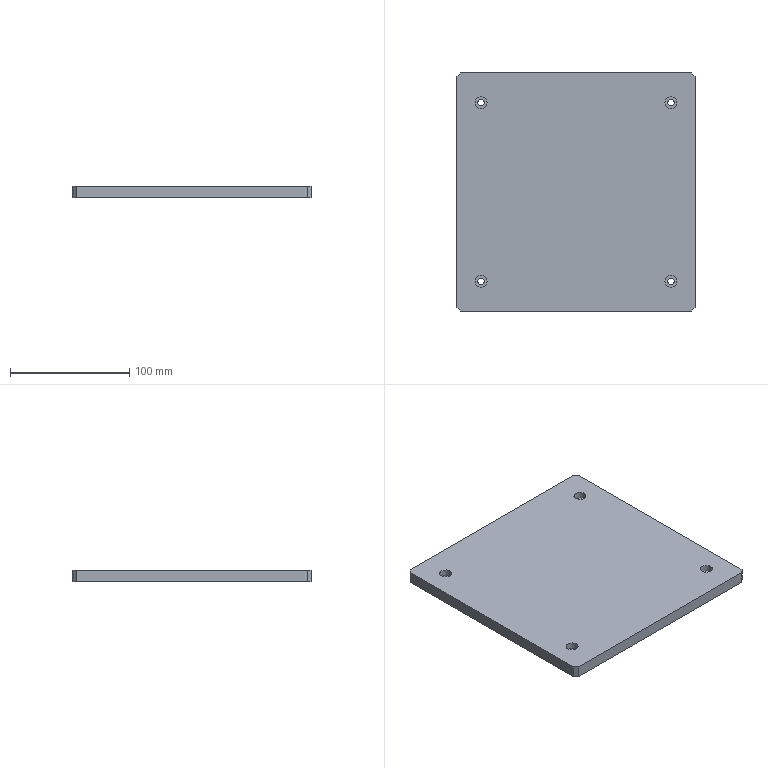Part | SolidWorks | features Chamfer 1, Extrusion 1, HoleWzd 1 | 1 solid | 30 faces | box 200 x 200 x 10 mm | volume 397621 mm3 | cylinder 16 | plane 14 | commonest cylinder face diameters 5.5 x8 10 x8
STEP:
#1=CARTESIAN_POINT('',(-84.68,75.,4.3));
#2=VERTEX_POINT('',#1);
#3=CARTESIAN_POINT('',(-74.68,75.,4.3));
#4=VERTEX_POINT('',#3);
#5=CARTESIAN_POINT('',(-79.68,75.,4.3));
#6=DIRECTION('',(0.,0.,1.));
#7=DIRECTION('',(1.,0.,0.));
#8=AXIS2_PLACEMENT_3D('',#5,#6,#7);
#9=CIRCLE('',#8,5.);
#10=EDGE_CURVE('',#2,#4,#9,.T.);
#11=ORIENTED_EDGE('',*,*,#10,.F.);
#12=CARTESIAN_POINT('',(-84.68,75.,10.));
#13=VERTEX_POINT('',#12);
#14=CARTESIAN_POINT('',(-84.68,75.,10.));
#15=DIRECTION('',(0.,0.,1.));
#16=VECTOR('',#15,1000.);
#17=LINE('',#14,#16);
#18=EDGE_CURVE('',#2,#13,#17,.T.);
#19=ORIENTED_EDGE('',*,*,#18,.T.);
#20=CARTESIAN_POINT('',(-74.68,75.,10.));
#21=VERTEX_POINT('',#20);
#22=CARTESIAN_POINT('',(-79.68,75.,10.));
#23=DIRECTION('',(0.,0.,1.));
#24=DIRECTION('',(1.,0.,0.));
#25=AXIS2_PLACEMENT_3D('',#22,#23,#24);
#26=CIRCLE('',#25,5.);
#27=EDGE_CURVE('',#13,#21,#26,.T.);
#28=ORIENTED_EDGE('',*,*,#27,.T.);
#29=CARTESIAN_POINT('',(-74.68,75.,10.));
#30=DIRECTION('',(0.,0.,1.));
#31=VECTOR('',#30,1000.);
#32=LINE('',#29,#31);
#33=EDGE_CURVE('',#4,#21,#32,.T.);
#34=ORIENTED_EDGE('',*,*,#33,.F.);
#35=EDGE_LOOP('',(#11,#19,#28,#34));
#36=FACE_OUTER_BOUND('',#35,.T.);
#37=CARTESIAN_POINT('',(-79.68,75.,10.));
#38=DIRECTION('',(0.,0.,1.));
#39=DIRECTION('',(1.,0.,0.));
#40=AXIS2_PLACEMENT_3D('',#37,#38,#39);
#41=CYLINDRICAL_SURFACE('',#40,5.);
#42=ADVANCED_FACE('',(#36),#41,.F.);
#43=CARTESIAN_POINT('',(-76.93,75.,0.));
#44=VERTEX_POINT('',#43);
#45=CARTESIAN_POINT('',(-82.43,75.,0.));
#46=VERTEX_POINT('',#45);
#47=CARTESIAN_POINT('',(-79.68,75.,0.));
#48=DIRECTION('',(0.,0.,-1.));
#49=DIRECTION('',(-1.,0.,0.));
#50=AXIS2_PLACEMENT_3D('',#47,#48,#49);
#51=CIRCLE('',#50,2.75);
#52=EDGE_CURVE('',#44,#46,#51,.T.);
#53=ORIENTED_EDGE('',*,*,#52,.T.);
#54=CARTESIAN_POINT('',(-82.43,75.,4.3));
#55=VERTEX_POINT('',#54);
#56=CARTESIAN_POINT('',(-82.43,75.,10.));
#57=DIRECTION('',(0.,0.,1.));
#58=VECTOR('',#57,1000.);
#59=LINE('',#56,#58);
#60=EDGE_CURVE('',#46,#55,#59,.T.);
#61=ORIENTED_EDGE('',*,*,#60,.T.);
#62=CARTESIAN_POINT('',(-76.93,75.,4.3));
#63=VERTEX_POINT('',#62);
#64=CARTESIAN_POINT('',(-79.68,75.,4.3));
#65=DIRECTION('',(0.,0.,1.));
#66=DIRECTION('',(1.,0.,0.));
#67=AXIS2_PLACEMENT_3D('',#64,#65,#66);
#68=CIRCLE('',#67,2.75);
#69=EDGE_CURVE('',#55,#63,#68,.T.);
#70=ORIENTED_EDGE('',*,*,#69,.T.);
#71=CARTESIAN_POINT('',(-76.93,75.,10.));
#72=DIRECTION('',(0.,0.,1.));
#73=VECTOR('',#72,1000.);
#74=LINE('',#71,#73);
#75=EDGE_CURVE('',#44,#63,#74,.T.);
#76=ORIENTED_EDGE('',*,*,#75,.F.);
#77=EDGE_LOOP('',(#53,#61,#70,#76));
#78=FACE_OUTER_BOUND('',#77,.T.);
#79=CARTESIAN_POINT('',(-79.68,75.,10.));
#80=DIRECTION('',(0.,0.,1.));
#81=DIRECTION('',(1.,0.,0.));
#82=AXIS2_PLACEMENT_3D('',#79,#80,#81);
#83=CYLINDRICAL_SURFACE('',#82,2.75);
#84=ADVANCED_FACE('',(#78),#83,.F.);
#85=CARTESIAN_POINT('',(74.68,75.,4.3));
#86=VERTEX_POINT('',#85);
#87=CARTESIAN_POINT('',(84.68,75.,4.3));
#88=VERTEX_POINT('',#87);
#89=CARTESIAN_POINT('',(79.68,75.,4.3));
#90=DIRECTION('',(0.,0.,1.));
#91=DIRECTION('',(1.,0.,0.));
#92=AXIS2_PLACEMENT_3D('',#89,#90,#91);
#93=CIRCLE('',#92,5.);
#94=EDGE_CURVE('',#86,#88,#93,.T.);
#95=ORIENTED_EDGE('',*,*,#94,.F.);
#96=CARTESIAN_POINT('',(74.68,75.,10.));
#97=VERTEX_POINT('',#96);
#98=CARTESIAN_POINT('',(74.68,75.,10.));
#99=DIRECTION('',(0.,0.,1.));
#100=VECTOR('',#99,1000.);
#101=LINE('',#98,#100);
#102=EDGE_CURVE('',#86,#97,#101,.T.);
#103=ORIENTED_EDGE('',*,*,#102,.T.);
#104=CARTESIAN_POINT('',(84.68,75.,10.));
#105=VERTEX_POINT('',#104);
#106=CARTESIAN_POINT('',(79.68,75.,10.));
#107=DIRECTION('',(0.,0.,1.));
#108=DIRECTION('',(1.,0.,0.));
#109=AXIS2_PLACEMENT_3D('',#106,#107,#108);
#110=CIRCLE('',#109,5.);
#111=EDGE_CURVE('',#97,#105,#110,.T.);
#112=ORIENTED_EDGE('',*,*,#111,.T.);
#113=CARTESIAN_POINT('',(84.68,75.,10.));
#114=DIRECTION('',(0.,0.,1.));
#115=VECTOR('',#114,1000.);
#116=LINE('',#113,#115);
#117=EDGE_CURVE('',#88,#105,#116,.T.);
#118=ORIENTED_EDGE('',*,*,#117,.F.);
#119=EDGE_LOOP('',(#95,#103,#112,#118));
#120=FACE_OUTER_BOUND('',#119,.T.);
#121=CARTESIAN_POINT('',(79.68,75.,10.));
#122=DIRECTION('',(0.,0.,1.));
#123=DIRECTION('',(1.,0.,0.));
#124=AXIS2_PLACEMENT_3D('',#121,#122,#123);
#125=CYLINDRICAL_SURFACE('',#124,5.);
#126=ADVANCED_FACE('',(#120),#125,.F.);
#127=CARTESIAN_POINT('',(82.43,75.,0.));
#128=VERTEX_POINT('',#127);
#129=CARTESIAN_POINT('',(76.93,75.,0.));
#130=VERTEX_POINT('',#129);
#131=CARTESIAN_POINT('',(79.68,75.,0.));
#132=DIRECTION('',(0.,0.,-1.));
#133=DIRECTION('',(-1.,0.,0.));
#134=AXIS2_PLACEMENT_3D('',#131,#132,#133);
#135=CIRCLE('',#134,2.75);
#136=EDGE_CURVE('',#128,#130,#135,.T.);
#137=ORIENTED_EDGE('',*,*,#136,.T.);
#138=CARTESIAN_POINT('',(76.93,75.,4.3));
#139=VERTEX_POINT('',#138);
#140=CARTESIAN_POINT('',(76.93,75.,10.));
#141=DIRECTION('',(0.,0.,1.));
#142=VECTOR('',#141,1000.);
#143=LINE('',#140,#142);
#144=EDGE_CURVE('',#130,#139,#143,.T.);
#145=ORIENTED_EDGE('',*,*,#144,.T.);
#146=CARTESIAN_POINT('',(82.43,75.,4.3));
#147=VERTEX_POINT('',#146);
#148=CARTESIAN_POINT('',(79.68,75.,4.3));
#149=DIRECTION('',(0.,0.,1.));
#150=DIRECTION('',(1.,0.,0.));
#151=AXIS2_PLACEMENT_3D('',#148,#149,#150);
#152=CIRCLE('',#151,2.75);
#153=EDGE_CURVE('',#139,#147,#152,.T.);
#154=ORIENTED_EDGE('',*,*,#153,.T.);
#155=CARTESIAN_POINT('',(82.43,75.,10.));
#156=DIRECTION('',(0.,0.,1.));
#157=VECTOR('',#156,1000.);
#158=LINE('',#155,#157);
#159=EDGE_CURVE('',#128,#147,#158,.T.);
#160=ORIENTED_EDGE('',*,*,#159,.F.);
#161=EDGE_LOOP('',(#137,#145,#154,#160));
#162=FACE_OUTER_BOUND('',#161,.T.);
#163=CARTESIAN_POINT('',(79.68,75.,10.));
#164=DIRECTION('',(0.,0.,1.));
#165=DIRECTION('',(1.,0.,0.));
#166=AXIS2_PLACEMENT_3D('',#163,#164,#165);
#167=CYLINDRICAL_SURFACE('',#166,2.75);
#168=ADVANCED_FACE('',(#162),#167,.F.);
#169=CARTESIAN_POINT('',(74.68,-75.,4.3));
#170=VERTEX_POINT('',#169);
#171=CARTESIAN_POINT('',(84.68,-75.,4.3));
#172=VERTEX_POINT('',#171);
#173=CARTESIAN_POINT('',(79.68,-75.,4.3));
#174=DIRECTION('',(0.,0.,1.));
#175=DIRECTION('',(1.,0.,0.));
#176=AXIS2_PLACEMENT_3D('',#173,#174,#175);
#177=CIRCLE('',#176,5.);
#178=EDGE_CURVE('',#170,#172,#177,.T.);
#179=ORIENTED_EDGE('',*,*,#178,.F.);
#180=CARTESIAN_POINT('',(74.68,-75.,10.));
#181=VERTEX_POINT('',#180);
#182=CARTESIAN_POINT('',(74.68,-75.,10.));
#183=DIRECTION('',(0.,0.,1.));
#184=VECTOR('',#183,1000.);
#185=LINE('',#182,#184);
#186=EDGE_CURVE('',#170,#181,#185,.T.);
#187=ORIENTED_EDGE('',*,*,#186,.T.);
#188=CARTESIAN_POINT('',(84.68,-75.,10.));
#189=VERTEX_POINT('',#188);
#190=CARTESIAN_POINT('',(79.68,-75.,10.));
#191=DIRECTION('',(0.,0.,1.));
#192=DIRECTION('',(1.,0.,0.));
#193=AXIS2_PLACEMENT_3D('',#190,#191,#192);
#194=CIRCLE('',#193,5.);
#195=EDGE_CURVE('',#181,#189,#194,.T.);
#196=ORIENTED_EDGE('',*,*,#195,.T.);
#197=CARTESIAN_POINT('',(84.68,-75.,10.));
#198=DIRECTION('',(0.,0.,1.));
#199=VECTOR('',#198,1000.);
#200=LINE('',#197,#199);
#201=EDGE_CURVE('',#172,#189,#200,.T.);
#202=ORIENTED_EDGE('',*,*,#201,.F.);
#203=EDGE_LOOP('',(#179,#187,#196,#202));
#204=FACE_OUTER_BOUND('',#203,.T.);
#205=CARTESIAN_POINT('',(79.68,-75.,10.));
#206=DIRECTION('',(0.,0.,1.));
#207=DIRECTION('',(1.,0.,0.));
#208=AXIS2_PLACEMENT_3D('',#205,#206,#207);
#209=CYLINDRICAL_SURFACE('',#208,5.);
#210=ADVANCED_FACE('',(#204),#209,.F.);
#211=CARTESIAN_POINT('',(82.43,-75.,0.));
#212=VERTEX_POINT('',#211);
#213=CARTESIAN_POINT('',(76.93,-75.,0.));
#214=VERTEX_POINT('',#213);
#215=CARTESIAN_POINT('',(79.68,-75.,0.));
#216=DIRECTION('',(0.,0.,-1.));
#217=DIRECTION('',(-1.,0.,0.));
#218=AXIS2_PLACEMENT_3D('',#215,#216,#217);
#219=CIRCLE('',#218,2.75);
#220=EDGE_CURVE('',#212,#214,#219,.T.);
#221=ORIENTED_EDGE('',*,*,#220,.T.);
#222=CARTESIAN_POINT('',(76.93,-75.,4.3));
#223=VERTEX_POINT('',#222);
#224=CARTESIAN_POINT('',(76.93,-75.,10.));
#225=DIRECTION('',(0.,0.,1.));
#226=VECTOR('',#225,1000.);
#227=LINE('',#224,#226);
#228=EDGE_CURVE('',#214,#223,#227,.T.);
#229=ORIENTED_EDGE('',*,*,#228,.T.);
#230=CARTESIAN_POINT('',(82.43,-75.,4.3));
#231=VERTEX_POINT('',#230);
#232=CARTESIAN_POINT('',(79.68,-75.,4.3));
#233=DIRECTION('',(0.,0.,1.));
#234=DIRECTION('',(1.,0.,0.));
#235=AXIS2_PLACEMENT_3D('',#232,#233,#234);
#236=CIRCLE('',#235,2.75);
#237=EDGE_CURVE('',#223,#231,#236,.T.);
#238=ORIENTED_EDGE('',*,*,#237,.T.);
#239=CARTESIAN_POINT('',(82.43,-75.,10.));
#240=DIRECTION('',(0.,0.,1.));
#241=VECTOR('',#240,1000.);
#242=LINE('',#239,#241);
#243=EDGE_CURVE('',#212,#231,#242,.T.);
#244=ORIENTED_EDGE('',*,*,#243,.F.);
#245=EDGE_LOOP('',(#221,#229,#238,#244));
#246=FACE_OUTER_BOUND('',#245,.T.);
#247=CARTESIAN_POINT('',(79.68,-75.,10.));
#248=DIRECTION('',(0.,0.,1.));
#249=DIRECTION('',(1.,0.,0.));
#250=AXIS2_PLACEMENT_3D('',#247,#248,#249);
#251=CYLINDRICAL_SURFACE('',#250,2.75);
#252=ADVANCED_FACE('',(#246),#251,.F.);
#253=CARTESIAN_POINT('',(-84.68,-75.,4.3));
#254=VERTEX_POINT('',#253);
#255=CARTESIAN_POINT('',(-74.68,-75.,4.3));
#256=VERTEX_POINT('',#255);
#257=CARTESIAN_POINT('',(-79.68,-75.,4.3));
#258=DIRECTION('',(0.,0.,1.));
#259=DIRECTION('',(1.,0.,0.));
#260=AXIS2_PLACEMENT_3D('',#257,#258,#259);
#261=CIRCLE('',#260,5.);
#262=EDGE_CURVE('',#254,#256,#261,.T.);
#263=ORIENTED_EDGE('',*,*,#262,.F.);
#264=CARTESIAN_POINT('',(-84.68,-75.,10.));
#265=VERTEX_POINT('',#264);
#266=CARTESIAN_POINT('',(-84.68,-75.,10.));
#267=DIRECTION('',(0.,0.,1.));
#268=VECTOR('',#267,1000.);
#269=LINE('',#266,#268);
#270=EDGE_CURVE('',#254,#265,#269,.T.);
#271=ORIENTED_EDGE('',*,*,#270,.T.);
#272=CARTESIAN_POINT('',(-74.68,-75.,10.));
#273=VERTEX_POINT('',#272);
#274=CARTESIAN_POINT('',(-79.68,-75.,10.));
#275=DIRECTION('',(0.,0.,1.));
#276=DIRECTION('',(1.,0.,0.));
#277=AXIS2_PLACEMENT_3D('',#274,#275,#276);
#278=CIRCLE('',#277,5.);
#279=EDGE_CURVE('',#265,#273,#278,.T.);
#280=ORIENTED_EDGE('',*,*,#279,.T.);
#281=CARTESIAN_POINT('',(-74.68,-75.,10.));
#282=DIRECTION('',(0.,0.,1.));
#283=VECTOR('',#282,1000.);
#284=LINE('',#281,#283);
#285=EDGE_CURVE('',#256,#273,#284,.T.);
#286=ORIENTED_EDGE('',*,*,#285,.F.);
#287=EDGE_LOOP('',(#263,#271,#280,#286));
#288=FACE_OUTER_BOUND('',#287,.T.);
#289=CARTESIAN_POINT('',(-79.68,-75.,10.));
#290=DIRECTION('',(0.,0.,1.));
#291=DIRECTION('',(1.,0.,0.));
#292=AXIS2_PLACEMENT_3D('',#289,#290,#291);
#293=CYLINDRICAL_SURFACE('',#292,5.);
#294=ADVANCED_FACE('',(#288),#293,.F.);
#295=CARTESIAN_POINT('',(-76.93,-75.,0.));
#296=VERTEX_POINT('',#295);
#297=CARTESIAN_POINT('',(-82.43,-75.,0.));
#298=VERTEX_POINT('',#297);
#299=CARTESIAN_POINT('',(-79.68,-75.,0.));
#300=DIRECTION('',(0.,0.,-1.));
#301=DIRECTION('',(-1.,0.,0.));
#302=AXIS2_PLACEMENT_3D('',#299,#300,#301);
#303=CIRCLE('',#302,2.75);
#304=EDGE_CURVE('',#296,#298,#303,.T.);
#305=ORIENTED_EDGE('',*,*,#304,.T.);
#306=CARTESIAN_POINT('',(-82.43,-75.,4.3));
#307=VERTEX_POINT('',#306);
#308=CARTESIAN_POINT('',(-82.43,-75.,10.));
#309=DIRECTION('',(0.,0.,1.));
#310=VECTOR('',#309,1000.);
#311=LINE('',#308,#310);
#312=EDGE_CURVE('',#298,#307,#311,.T.);
#313=ORIENTED_EDGE('',*,*,#312,.T.);
#314=CARTESIAN_POINT('',(-76.93,-75.,4.3));
#315=VERTEX_POINT('',#314);
#316=CARTESIAN_POINT('',(-79.68,-75.,4.3));
#317=DIRECTION('',(0.,0.,1.));
#318=DIRECTION('',(1.,0.,0.));
#319=AXIS2_PLACEMENT_3D('',#316,#317,#318);
#320=CIRCLE('',#319,2.75);
#321=EDGE_CURVE('',#307,#315,#320,.T.);
#322=ORIENTED_EDGE('',*,*,#321,.T.);
#323=CARTESIAN_POINT('',(-76.93,-75.,10.));
#324=DIRECTION('',(0.,0.,1.));
#325=VECTOR('',#324,1000.);
#326=LINE('',#323,#325);
#327=EDGE_CURVE('',#296,#315,#326,.T.);
#328=ORIENTED_EDGE('',*,*,#327,.F.);
#329=EDGE_LOOP('',(#305,#313,#322,#328));
#330=FACE_OUTER_BOUND('',#329,.T.);
#331=CARTESIAN_POINT('',(-79.68,-75.,10.));
#332=DIRECTION('',(0.,0.,1.));
#333=DIRECTION('',(1.,0.,0.));
#334=AXIS2_PLACEMENT_3D('',#331,#332,#333);
#335=CYLINDRICAL_SURFACE('',#334,2.75);
#336=ADVANCED_FACE('',(#330),#335,.F.);
#337=CARTESIAN_POINT('',(100.,-97.,0.));
#338=VERTEX_POINT('',#337);
#339=CARTESIAN_POINT('',(100.,97.,0.));
#340=VERTEX_POINT('',#339);
#341=CARTESIAN_POINT('',(100.,-100.,0.));
#342=DIRECTION('',(0.,1.,0.));
#343=VECTOR('',#342,1000.);
#344=LINE('',#341,#343);
#345=EDGE_CURVE('',#338,#340,#344,.T.);
#346=ORIENTED_EDGE('',*,*,#345,.T.);
#347=CARTESIAN_POINT('',(100.,97.,10.));
#348=VERTEX_POINT('',#347);
#349=CARTESIAN_POINT('',(100.,97.,10.));
#350=DIRECTION('',(0.,0.,1.));
#351=VECTOR('',#350,1000.);
#352=LINE('',#349,#351);
#353=EDGE_CURVE('',#340,#348,#352,.T.);
#354=ORIENTED_EDGE('',*,*,#353,.T.);
#355=CARTESIAN_POINT('',(100.,-97.,10.));
#356=VERTEX_POINT('',#355);
#357=CARTESIAN_POINT('',(100.,-100.,10.));
#358=DIRECTION('',(0.,1.,0.));
#359=VECTOR('',#358,1000.);
#360=LINE('',#357,#359);
#361=EDGE_CURVE('',#356,#348,#360,.T.);
#362=ORIENTED_EDGE('',*,*,#361,.F.);
#363=CARTESIAN_POINT('',(100.,-97.,10.));
#364=DIRECTION('',(0.,0.,-1.));
#365=VECTOR('',#364,1000.);
#366=LINE('',#363,#365);
#367=EDGE_CURVE('',#356,#338,#366,.T.);
#368=ORIENTED_EDGE('',*,*,#367,.T.);
#369=EDGE_LOOP('',(#346,#354,#362,#368));
#370=FACE_OUTER_BOUND('',#369,.T.);
#371=CARTESIAN_POINT('',(100.,-100.,10.));
#372=DIRECTION('',(-1.,0.,0.));
#373=DIRECTION('',(0.,0.,1.));
#374=AXIS2_PLACEMENT_3D('',#371,#372,#373);
#375=PLANE('',#374);
#376=ADVANCED_FACE('',(#370),#375,.F.);
#377=CARTESIAN_POINT('',(97.,100.,0.));
#378=VERTEX_POINT('',#377);
#379=CARTESIAN_POINT('',(-97.,100.,0.));
#380=VERTEX_POINT('',#379);
#381=CARTESIAN_POINT('',(-100.,100.,0.));
#382=DIRECTION('',(-1.,0.,0.));
#383=VECTOR('',#382,1000.);
#384=LINE('',#381,#383);
#385=EDGE_CURVE('',#378,#380,#384,.T.);
#386=ORIENTED_EDGE('',*,*,#385,.T.);
#387=CARTESIAN_POINT('',(-97.,100.,10.));
#388=VERTEX_POINT('',#387);
#389=CARTESIAN_POINT('',(-97.,100.,10.));
#390=DIRECTION('',(0.,0.,1.));
#391=VECTOR('',#390,1000.);
#392=LINE('',#389,#391);
#393=EDGE_CURVE('',#380,#388,#392,.T.);
#394=ORIENTED_EDGE('',*,*,#393,.T.);
#395=CARTESIAN_POINT('',(97.,100.,10.));
#396=VERTEX_POINT('',#395);
#397=CARTESIAN_POINT('',(-100.,100.,10.));
#398=DIRECTION('',(-1.,0.,0.));
#399=VECTOR('',#398,1000.);
#400=LINE('',#397,#399);
#401=EDGE_CURVE('',#396,#388,#400,.T.);
#402=ORIENTED_EDGE('',*,*,#401,.F.);
#403=CARTESIAN_POINT('',(97.,100.,10.));
#404=DIRECTION('',(0.,0.,-1.));
#405=VECTOR('',#404,1000.);
#406=LINE('',#403,#405);
#407=EDGE_CURVE('',#396,#378,#406,.T.);
#408=ORIENTED_EDGE('',*,*,#407,.T.);
#409=EDGE_LOOP('',(#386,#394,#402,#408));
#410=FACE_OUTER_BOUND('',#409,.T.);
#411=CARTESIAN_POINT('',(-100.,100.,10.));
#412=DIRECTION('',(0.,-1.,0.));
#413=DIRECTION('',(0.,0.,-1.));
#414=AXIS2_PLACEMENT_3D('',#411,#412,#413);
#415=PLANE('',#414);
#416=ADVANCED_FACE('',(#410),#415,.F.);
#417=CARTESIAN_POINT('',(-100.,97.,10.));
#418=VERTEX_POINT('',#417);
#419=CARTESIAN_POINT('',(-100.,-97.,10.));
#420=VERTEX_POINT('',#419);
#421=CARTESIAN_POINT('',(-100.,-100.,10.));
#422=DIRECTION('',(0.,-1.,0.));
#423=VECTOR('',#422,1000.);
#424=LINE('',#421,#423);
#425=EDGE_CURVE('',#418,#420,#424,.T.);
#426=ORIENTED_EDGE('',*,*,#425,.F.);
#427=CARTESIAN_POINT('',(-100.,97.,0.));
#428=VERTEX_POINT('',#427);
#429=CARTESIAN_POINT('',(-100.,97.,10.));
#430=DIRECTION('',(0.,0.,-1.));
#431=VECTOR('',#430,1000.);
#432=LINE('',#429,#431);
#433=EDGE_CURVE('',#418,#428,#432,.T.);
#434=ORIENTED_EDGE('',*,*,#433,.T.);
#435=CARTESIAN_POINT('',(-100.,-97.,0.));
#436=VERTEX_POINT('',#435);
#437=CARTESIAN_POINT('',(-100.,-100.,0.));
#438=DIRECTION('',(0.,-1.,0.));
#439=VECTOR('',#438,1000.);
#440=LINE('',#437,#439);
#441=EDGE_CURVE('',#428,#436,#440,.T.);
#442=ORIENTED_EDGE('',*,*,#441,.T.);
#443=CARTESIAN_POINT('',(-100.,-97.,10.));
#444=DIRECTION('',(0.,0.,1.));
#445=VECTOR('',#444,1000.);
#446=LINE('',#443,#445);
#447=EDGE_CURVE('',#436,#420,#446,.T.);
#448=ORIENTED_EDGE('',*,*,#447,.T.);
#449=EDGE_LOOP('',(#426,#434,#442,#448));
#450=FACE_OUTER_BOUND('',#449,.T.);
#451=CARTESIAN_POINT('',(-100.,-100.,10.));
#452=DIRECTION('',(1.,0.,0.));
#453=DIRECTION('',(0.,0.,-1.));
#454=AXIS2_PLACEMENT_3D('',#451,#452,#453);
#455=PLANE('',#454);
#456=ADVANCED_FACE('',(#450),#455,.F.);
#457=CARTESIAN_POINT('',(-97.,-100.,10.));
#458=VERTEX_POINT('',#457);
#459=CARTESIAN_POINT('',(97.,-100.,10.));
#460=VERTEX_POINT('',#459);
#461=CARTESIAN_POINT('',(-100.,-100.,10.));
#462=DIRECTION('',(1.,0.,0.));
#463=VECTOR('',#462,1000.);
#464=LINE('',#461,#463);
#465=EDGE_CURVE('',#458,#460,#464,.T.);
#466=ORIENTED_EDGE('',*,*,#465,.F.);
#467=CARTESIAN_POINT('',(-97.,-100.,0.));
#468=VERTEX_POINT('',#467);
#469=CARTESIAN_POINT('',(-97.,-100.,10.));
#470=DIRECTION('',(0.,0.,-1.));
#471=VECTOR('',#470,1000.);
#472=LINE('',#469,#471);
#473=EDGE_CURVE('',#458,#468,#472,.T.);
#474=ORIENTED_EDGE('',*,*,#473,.T.);
#475=CARTESIAN_POINT('',(97.,-100.,0.));
#476=VERTEX_POINT('',#475);
#477=CARTESIAN_POINT('',(-100.,-100.,0.));
#478=DIRECTION('',(1.,0.,0.));
#479=VECTOR('',#478,1000.);
#480=LINE('',#477,#479);
#481=EDGE_CURVE('',#468,#476,#480,.T.);
#482=ORIENTED_EDGE('',*,*,#481,.T.);
#483=CARTESIAN_POINT('',(97.,-100.,10.));
#484=DIRECTION('',(0.,0.,1.));
#485=VECTOR('',#484,1000.);
#486=LINE('',#483,#485);
#487=EDGE_CURVE('',#476,#460,#486,.T.);
#488=ORIENTED_EDGE('',*,*,#487,.T.);
#489=EDGE_LOOP('',(#466,#474,#482,#488));
#490=FACE_OUTER_BOUND('',#489,.T.);
#491=CARTESIAN_POINT('',(-100.,-100.,10.));
#492=DIRECTION('',(0.,1.,0.));
#493=DIRECTION('',(0.,0.,1.));
#494=AXIS2_PLACEMENT_3D('',#491,#492,#493);
#495=PLANE('',#494);
#496=ADVANCED_FACE('',(#490),#495,.F.);
#497=CARTESIAN_POINT('',(-79.68,75.,10.));
#498=DIRECTION('',(0.,0.,1.));
#499=DIRECTION('',(1.,0.,0.));
#500=AXIS2_PLACEMENT_3D('',#497,#498,#499);
#501=CIRCLE('',#500,5.);
#502=EDGE_CURVE('',#21,#13,#501,.T.);
#503=ORIENTED_EDGE('',*,*,#502,.F.);
#504=ORIENTED_EDGE('',*,*,#27,.F.);
#505=EDGE_LOOP('',(#503,#504));
#506=FACE_BOUND('',#505,.T.);
#507=CARTESIAN_POINT('',(79.68,75.,10.));
#508=DIRECTION('',(0.,0.,1.));
#509=DIRECTION('',(1.,0.,0.));
#510=AXIS2_PLACEMENT_3D('',#507,#508,#509);
#511=CIRCLE('',#510,5.);
#512=EDGE_CURVE('',#105,#97,#511,.T.);
#513=ORIENTED_EDGE('',*,*,#512,.F.);
#514=ORIENTED_EDGE('',*,*,#111,.F.);
#515=EDGE_LOOP('',(#513,#514));
#516=FACE_BOUND('',#515,.T.);
#517=CARTESIAN_POINT('',(79.68,-75.,10.));
#518=DIRECTION('',(0.,0.,1.));
#519=DIRECTION('',(1.,0.,0.));
#520=AXIS2_PLACEMENT_3D('',#517,#518,#519);
#521=CIRCLE('',#520,5.);
#522=EDGE_CURVE('',#189,#181,#521,.T.);
#523=ORIENTED_EDGE('',*,*,#522,.F.);
#524=ORIENTED_EDGE('',*,*,#195,.F.);
#525=EDGE_LOOP('',(#523,#524));
#526=FACE_BOUND('',#525,.T.);
#527=CARTESIAN_POINT('',(-79.68,-75.,10.));
#528=DIRECTION('',(0.,0.,1.));
#529=DIRECTION('',(1.,0.,0.));
#530=AXIS2_PLACEMENT_3D('',#527,#528,#529);
#531=CIRCLE('',#530,5.);
#532=EDGE_CURVE('',#273,#265,#531,.T.);
#533=ORIENTED_EDGE('',*,*,#532,.F.);
#534=ORIENTED_EDGE('',*,*,#279,.F.);
#535=EDGE_LOOP('',(#533,#534));
#536=FACE_BOUND('',#535,.T.);
#537=ORIENTED_EDGE('',*,*,#401,.T.);
#538=CARTESIAN_POINT('',(-100.,97.,10.));
#539=DIRECTION('',(-0.7071,-0.7071,0.));
#540=VECTOR('',#539,1000.);
#541=LINE('',#538,#540);
#542=EDGE_CURVE('',#388,#418,#541,.T.);
#543=ORIENTED_EDGE('',*,*,#542,.T.);
#544=ORIENTED_EDGE('',*,*,#425,.T.);
#545=CARTESIAN_POINT('',(-97.,-100.,10.));
#546=DIRECTION('',(0.7071,-0.7071,0.));
#547=VECTOR('',#546,1000.);
#548=LINE('',#545,#547);
#549=EDGE_CURVE('',#420,#458,#548,.T.);
#550=ORIENTED_EDGE('',*,*,#549,.T.);
#551=ORIENTED_EDGE('',*,*,#465,.T.);
#552=CARTESIAN_POINT('',(100.,-97.,10.));
#553=DIRECTION('',(0.7071,0.7071,0.));
#554=VECTOR('',#553,1000.);
#555=LINE('',#552,#554);
#556=EDGE_CURVE('',#460,#356,#555,.T.);
#557=ORIENTED_EDGE('',*,*,#556,.T.);
#558=ORIENTED_EDGE('',*,*,#361,.T.);
#559=CARTESIAN_POINT('',(97.,100.,10.));
#560=DIRECTION('',(-0.7071,0.7071,0.));
#561=VECTOR('',#560,1000.);
#562=LINE('',#559,#561);
#563=EDGE_CURVE('',#348,#396,#562,.T.);
#564=ORIENTED_EDGE('',*,*,#563,.T.);
#565=EDGE_LOOP('',(#537,#543,#544,#550,#551,#557,#558,#564));
#566=FACE_OUTER_BOUND('',#565,.T.);
#567=CARTESIAN_POINT('',(0.,0.,10.));
#568=DIRECTION('',(0.,0.,-1.));
#569=DIRECTION('',(-1.,0.,0.));
#570=AXIS2_PLACEMENT_3D('',#567,#568,#569);
#571=PLANE('',#570);
#572=ADVANCED_FACE('',(#506,#516,#526,#536,#566),#571,.F.);
#573=ORIENTED_EDGE('',*,*,#52,.F.);
#574=CARTESIAN_POINT('',(-79.68,75.,0.));
#575=DIRECTION('',(0.,0.,-1.));
#576=DIRECTION('',(-1.,0.,0.));
#577=AXIS2_PLACEMENT_3D('',#574,#575,#576);
#578=CIRCLE('',#577,2.75);
#579=EDGE_CURVE('',#46,#44,#578,.T.);
#580=ORIENTED_EDGE('',*,*,#579,.F.);
#581=EDGE_LOOP('',(#573,#580));
#582=FACE_BOUND('',#581,.T.);
#583=ORIENTED_EDGE('',*,*,#136,.F.);
#584=CARTESIAN_POINT('',(79.68,75.,0.));
#585=DIRECTION('',(0.,0.,-1.));
#586=DIRECTION('',(-1.,0.,0.));
#587=AXIS2_PLACEMENT_3D('',#584,#585,#586);
#588=CIRCLE('',#587,2.75);
#589=EDGE_CURVE('',#130,#128,#588,.T.);
#590=ORIENTED_EDGE('',*,*,#589,.F.);
#591=EDGE_LOOP('',(#583,#590));
#592=FACE_BOUND('',#591,.T.);
#593=ORIENTED_EDGE('',*,*,#220,.F.);
#594=CARTESIAN_POINT('',(79.68,-75.,0.));
#595=DIRECTION('',(0.,0.,-1.));
#596=DIRECTION('',(-1.,0.,0.));
#597=AXIS2_PLACEMENT_3D('',#594,#595,#596);
#598=CIRCLE('',#597,2.75);
#599=EDGE_CURVE('',#214,#212,#598,.T.);
#600=ORIENTED_EDGE('',*,*,#599,.F.);
#601=EDGE_LOOP('',(#593,#600));
#602=FACE_BOUND('',#601,.T.);
#603=ORIENTED_EDGE('',*,*,#304,.F.);
#604=CARTESIAN_POINT('',(-79.68,-75.,0.));
#605=DIRECTION('',(0.,0.,-1.));
#606=DIRECTION('',(-1.,0.,0.));
#607=AXIS2_PLACEMENT_3D('',#604,#605,#606);
#608=CIRCLE('',#607,2.75);
#609=EDGE_CURVE('',#298,#296,#608,.T.);
#610=ORIENTED_EDGE('',*,*,#609,.F.);
#611=EDGE_LOOP('',(#603,#610));
#612=FACE_BOUND('',#611,.T.);
#613=ORIENTED_EDGE('',*,*,#441,.F.);
#614=CARTESIAN_POINT('',(-98.5,98.5,0.));
#615=DIRECTION('',(0.7071,0.7071,0.));
#616=VECTOR('',#615,1000.);
#617=LINE('',#614,#616);
#618=EDGE_CURVE('',#428,#380,#617,.T.);
#619=ORIENTED_EDGE('',*,*,#618,.T.);
#620=ORIENTED_EDGE('',*,*,#385,.F.);
#621=CARTESIAN_POINT('',(98.5,98.5,0.));
#622=DIRECTION('',(0.7071,-0.7071,0.));
#623=VECTOR('',#622,1000.);
#624=LINE('',#621,#623);
#625=EDGE_CURVE('',#378,#340,#624,.T.);
#626=ORIENTED_EDGE('',*,*,#625,.T.);
#627=ORIENTED_EDGE('',*,*,#345,.F.);
#628=CARTESIAN_POINT('',(98.5,-98.5,0.));
#629=DIRECTION('',(-0.7071,-0.7071,0.));
#630=VECTOR('',#629,1000.);
#631=LINE('',#628,#630);
#632=EDGE_CURVE('',#338,#476,#631,.T.);
#633=ORIENTED_EDGE('',*,*,#632,.T.);
#634=ORIENTED_EDGE('',*,*,#481,.F.);
#635=CARTESIAN_POINT('',(-98.5,-98.5,0.));
#636=DIRECTION('',(-0.7071,0.7071,0.));
#637=VECTOR('',#636,1000.);
#638=LINE('',#635,#637);
#639=EDGE_CURVE('',#468,#436,#638,.T.);
#640=ORIENTED_EDGE('',*,*,#639,.T.);
#641=EDGE_LOOP('',(#613,#619,#620,#626,#627,#633,#634,#640));
#642=FACE_OUTER_BOUND('',#641,.T.);
#643=CARTESIAN_POINT('',(0.,0.,0.));
#644=DIRECTION('',(0.,0.,-1.));
#645=DIRECTION('',(-1.,0.,0.));
#646=AXIS2_PLACEMENT_3D('',#643,#644,#645);
#647=PLANE('',#646);
#648=ADVANCED_FACE('',(#582,#592,#602,#612,#642),#647,.T.);
#649=ORIENTED_EDGE('',*,*,#312,.F.);
#650=ORIENTED_EDGE('',*,*,#609,.T.);
#651=ORIENTED_EDGE('',*,*,#327,.T.);
#652=CARTESIAN_POINT('',(-79.68,-75.,4.3));
#653=DIRECTION('',(0.,0.,1.));
#654=DIRECTION('',(1.,0.,0.));
#655=AXIS2_PLACEMENT_3D('',#652,#653,#654);
#656=CIRCLE('',#655,2.75);
#657=EDGE_CURVE('',#315,#307,#656,.T.);
#658=ORIENTED_EDGE('',*,*,#657,.T.);
#659=EDGE_LOOP('',(#649,#650,#651,#658));
#660=FACE_OUTER_BOUND('',#659,.T.);
#661=CARTESIAN_POINT('',(-79.68,-75.,10.));
#662=DIRECTION('',(0.,0.,1.));
#663=DIRECTION('',(1.,0.,0.));
#664=AXIS2_PLACEMENT_3D('',#661,#662,#663);
#665=CYLINDRICAL_SURFACE('',#664,2.75);
#666=ADVANCED_FACE('',(#660),#665,.F.);
#667=ORIENTED_EDGE('',*,*,#657,.F.);
#668=ORIENTED_EDGE('',*,*,#321,.F.);
#669=EDGE_LOOP('',(#667,#668));
#670=FACE_BOUND('',#669,.T.);
#671=CARTESIAN_POINT('',(-79.68,-75.,4.3));
#672=DIRECTION('',(0.,0.,1.));
#673=DIRECTION('',(1.,0.,0.));
#674=AXIS2_PLACEMENT_3D('',#671,#672,#673);
#675=CIRCLE('',#674,5.);
#676=EDGE_CURVE('',#256,#254,#675,.T.);
#677=ORIENTED_EDGE('',*,*,#676,.T.);
#678=ORIENTED_EDGE('',*,*,#262,.T.);
#679=EDGE_LOOP('',(#677,#678));
#680=FACE_OUTER_BOUND('',#679,.T.);
#681=CARTESIAN_POINT('',(-76.93,-75.,4.3));
#682=DIRECTION('',(0.,0.,-1.));
#683=DIRECTION('',(-1.,0.,0.));
#684=AXIS2_PLACEMENT_3D('',#681,#682,#683);
#685=PLANE('',#684);
#686=ADVANCED_FACE('',(#670,#680),#685,.F.);
#687=ORIENTED_EDGE('',*,*,#270,.F.);
#688=ORIENTED_EDGE('',*,*,#676,.F.);
#689=ORIENTED_EDGE('',*,*,#285,.T.);
#690=ORIENTED_EDGE('',*,*,#532,.T.);
#691=EDGE_LOOP('',(#687,#688,#689,#690));
#692=FACE_OUTER_BOUND('',#691,.T.);
#693=CARTESIAN_POINT('',(-79.68,-75.,10.));
#694=DIRECTION('',(0.,0.,1.));
#695=DIRECTION('',(1.,0.,0.));
#696=AXIS2_PLACEMENT_3D('',#693,#694,#695);
#697=CYLINDRICAL_SURFACE('',#696,5.);
#698=ADVANCED_FACE('',(#692),#697,.F.);
#699=ORIENTED_EDGE('',*,*,#228,.F.);
#700=ORIENTED_EDGE('',*,*,#599,.T.);
#701=ORIENTED_EDGE('',*,*,#243,.T.);
#702=CARTESIAN_POINT('',(79.68,-75.,4.3));
#703=DIRECTION('',(0.,0.,1.));
#704=DIRECTION('',(1.,0.,0.));
#705=AXIS2_PLACEMENT_3D('',#702,#703,#704);
#706=CIRCLE('',#705,2.75);
#707=EDGE_CURVE('',#231,#223,#706,.T.);
#708=ORIENTED_EDGE('',*,*,#707,.T.);
#709=EDGE_LOOP('',(#699,#700,#701,#708));
#710=FACE_OUTER_BOUND('',#709,.T.);
#711=CARTESIAN_POINT('',(79.68,-75.,10.));
#712=DIRECTION('',(0.,0.,1.));
#713=DIRECTION('',(1.,0.,0.));
#714=AXIS2_PLACEMENT_3D('',#711,#712,#713);
#715=CYLINDRICAL_SURFACE('',#714,2.75);
#716=ADVANCED_FACE('',(#710),#715,.F.);
#717=ORIENTED_EDGE('',*,*,#707,.F.);
#718=ORIENTED_EDGE('',*,*,#237,.F.);
#719=EDGE_LOOP('',(#717,#718));
#720=FACE_BOUND('',#719,.T.);
#721=CARTESIAN_POINT('',(79.68,-75.,4.3));
#722=DIRECTION('',(0.,0.,1.));
#723=DIRECTION('',(1.,0.,0.));
#724=AXIS2_PLACEMENT_3D('',#721,#722,#723);
#725=CIRCLE('',#724,5.);
#726=EDGE_CURVE('',#172,#170,#725,.T.);
#727=ORIENTED_EDGE('',*,*,#726,.T.);
#728=ORIENTED_EDGE('',*,*,#178,.T.);
#729=EDGE_LOOP('',(#727,#728));
#730=FACE_OUTER_BOUND('',#729,.T.);
#731=CARTESIAN_POINT('',(82.43,-75.,4.3));
#732=DIRECTION('',(0.,0.,-1.));
#733=DIRECTION('',(-1.,0.,0.));
#734=AXIS2_PLACEMENT_3D('',#731,#732,#733);
#735=PLANE('',#734);
#736=ADVANCED_FACE('',(#720,#730),#735,.F.);
#737=ORIENTED_EDGE('',*,*,#186,.F.);
#738=ORIENTED_EDGE('',*,*,#726,.F.);
#739=ORIENTED_EDGE('',*,*,#201,.T.);
#740=ORIENTED_EDGE('',*,*,#522,.T.);
#741=EDGE_LOOP('',(#737,#738,#739,#740));
#742=FACE_OUTER_BOUND('',#741,.T.);
#743=CARTESIAN_POINT('',(79.68,-75.,10.));
#744=DIRECTION('',(0.,0.,1.));
#745=DIRECTION('',(1.,0.,0.));
#746=AXIS2_PLACEMENT_3D('',#743,#744,#745);
#747=CYLINDRICAL_SURFACE('',#746,5.);
#748=ADVANCED_FACE('',(#742),#747,.F.);
#749=ORIENTED_EDGE('',*,*,#144,.F.);
#750=ORIENTED_EDGE('',*,*,#589,.T.);
#751=ORIENTED_EDGE('',*,*,#159,.T.);
#752=CARTESIAN_POINT('',(79.68,75.,4.3));
#753=DIRECTION('',(0.,0.,1.));
#754=DIRECTION('',(1.,0.,0.));
#755=AXIS2_PLACEMENT_3D('',#752,#753,#754);
#756=CIRCLE('',#755,2.75);
#757=EDGE_CURVE('',#147,#139,#756,.T.);
#758=ORIENTED_EDGE('',*,*,#757,.T.);
#759=EDGE_LOOP('',(#749,#750,#751,#758));
#760=FACE_OUTER_BOUND('',#759,.T.);
#761=CARTESIAN_POINT('',(79.68,75.,10.));
#762=DIRECTION('',(0.,0.,1.));
#763=DIRECTION('',(1.,0.,0.));
#764=AXIS2_PLACEMENT_3D('',#761,#762,#763);
#765=CYLINDRICAL_SURFACE('',#764,2.75);
#766=ADVANCED_FACE('',(#760),#765,.F.);
#767=ORIENTED_EDGE('',*,*,#757,.F.);
#768=ORIENTED_EDGE('',*,*,#153,.F.);
#769=EDGE_LOOP('',(#767,#768));
#770=FACE_BOUND('',#769,.T.);
#771=CARTESIAN_POINT('',(79.68,75.,4.3));
#772=DIRECTION('',(0.,0.,1.));
#773=DIRECTION('',(1.,0.,0.));
#774=AXIS2_PLACEMENT_3D('',#771,#772,#773);
#775=CIRCLE('',#774,5.);
#776=EDGE_CURVE('',#88,#86,#775,.T.);
#777=ORIENTED_EDGE('',*,*,#776,.T.);
#778=ORIENTED_EDGE('',*,*,#94,.T.);
#779=EDGE_LOOP('',(#777,#778));
#780=FACE_OUTER_BOUND('',#779,.T.);
#781=CARTESIAN_POINT('',(82.43,75.,4.3));
#782=DIRECTION('',(0.,0.,-1.));
#783=DIRECTION('',(-1.,0.,0.));
#784=AXIS2_PLACEMENT_3D('',#781,#782,#783);
#785=PLANE('',#784);
#786=ADVANCED_FACE('',(#770,#780),#785,.F.);
#787=ORIENTED_EDGE('',*,*,#102,.F.);
#788=ORIENTED_EDGE('',*,*,#776,.F.);
#789=ORIENTED_EDGE('',*,*,#117,.T.);
#790=ORIENTED_EDGE('',*,*,#512,.T.);
#791=EDGE_LOOP('',(#787,#788,#789,#790));
#792=FACE_OUTER_BOUND('',#791,.T.);
#793=CARTESIAN_POINT('',(79.68,75.,10.));
#794=DIRECTION('',(0.,0.,1.));
#795=DIRECTION('',(1.,0.,0.));
#796=AXIS2_PLACEMENT_3D('',#793,#794,#795);
#797=CYLINDRICAL_SURFACE('',#796,5.);
#798=ADVANCED_FACE('',(#792),#797,.F.);
#799=ORIENTED_EDGE('',*,*,#60,.F.);
#800=ORIENTED_EDGE('',*,*,#579,.T.);
#801=ORIENTED_EDGE('',*,*,#75,.T.);
#802=CARTESIAN_POINT('',(-79.68,75.,4.3));
#803=DIRECTION('',(0.,0.,1.));
#804=DIRECTION('',(1.,0.,0.));
#805=AXIS2_PLACEMENT_3D('',#802,#803,#804);
#806=CIRCLE('',#805,2.75);
#807=EDGE_CURVE('',#63,#55,#806,.T.);
#808=ORIENTED_EDGE('',*,*,#807,.T.);
#809=EDGE_LOOP('',(#799,#800,#801,#808));
#810=FACE_OUTER_BOUND('',#809,.T.);
#811=CARTESIAN_POINT('',(-79.68,75.,10.));
#812=DIRECTION('',(0.,0.,1.));
#813=DIRECTION('',(1.,0.,0.));
#814=AXIS2_PLACEMENT_3D('',#811,#812,#813);
#815=CYLINDRICAL_SURFACE('',#814,2.75);
#816=ADVANCED_FACE('',(#810),#815,.F.);
#817=ORIENTED_EDGE('',*,*,#807,.F.);
#818=ORIENTED_EDGE('',*,*,#69,.F.);
#819=EDGE_LOOP('',(#817,#818));
#820=FACE_BOUND('',#819,.T.);
#821=CARTESIAN_POINT('',(-79.68,75.,4.3));
#822=DIRECTION('',(0.,0.,1.));
#823=DIRECTION('',(1.,0.,0.));
#824=AXIS2_PLACEMENT_3D('',#821,#822,#823);
#825=CIRCLE('',#824,5.);
#826=EDGE_CURVE('',#4,#2,#825,.T.);
#827=ORIENTED_EDGE('',*,*,#826,.T.);
#828=ORIENTED_EDGE('',*,*,#10,.T.);
#829=EDGE_LOOP('',(#827,#828));
#830=FACE_OUTER_BOUND('',#829,.T.);
#831=CARTESIAN_POINT('',(-76.93,75.,4.3));
#832=DIRECTION('',(0.,0.,-1.));
#833=DIRECTION('',(-1.,0.,0.));
#834=AXIS2_PLACEMENT_3D('',#831,#832,#833);
#835=PLANE('',#834);
#836=ADVANCED_FACE('',(#820,#830),#835,.F.);
#837=ORIENTED_EDGE('',*,*,#18,.F.);
#838=ORIENTED_EDGE('',*,*,#826,.F.);
#839=ORIENTED_EDGE('',*,*,#33,.T.);
#840=ORIENTED_EDGE('',*,*,#502,.T.);
#841=EDGE_LOOP('',(#837,#838,#839,#840));
#842=FACE_OUTER_BOUND('',#841,.T.);
#843=CARTESIAN_POINT('',(-79.68,75.,10.));
#844=DIRECTION('',(0.,0.,1.));
#845=DIRECTION('',(1.,0.,0.));
#846=AXIS2_PLACEMENT_3D('',#843,#844,#845);
#847=CYLINDRICAL_SURFACE('',#846,5.);
#848=ADVANCED_FACE('',(#842),#847,.F.);
#849=ORIENTED_EDGE('',*,*,#542,.F.);
#850=ORIENTED_EDGE('',*,*,#393,.F.);
#851=ORIENTED_EDGE('',*,*,#618,.F.);
#852=ORIENTED_EDGE('',*,*,#433,.F.);
#853=EDGE_LOOP('',(#849,#850,#851,#852));
#854=FACE_OUTER_BOUND('',#853,.T.);
#855=CARTESIAN_POINT('',(-100.,97.,10.));
#856=DIRECTION('',(0.7071,-0.7071,0.));
#857=DIRECTION('',(0.,0.,-1.));
#858=AXIS2_PLACEMENT_3D('',#855,#856,#857);
#859=PLANE('',#858);
#860=ADVANCED_FACE('',(#854),#859,.F.);
#861=ORIENTED_EDGE('',*,*,#563,.F.);
#862=ORIENTED_EDGE('',*,*,#353,.F.);
#863=ORIENTED_EDGE('',*,*,#625,.F.);
#864=ORIENTED_EDGE('',*,*,#407,.F.);
#865=EDGE_LOOP('',(#861,#862,#863,#864));
#866=FACE_OUTER_BOUND('',#865,.T.);
#867=CARTESIAN_POINT('',(97.,100.,10.));
#868=DIRECTION('',(-0.7071,-0.7071,0.));
#869=DIRECTION('',(0.,0.,-1.));
#870=AXIS2_PLACEMENT_3D('',#867,#868,#869);
#871=PLANE('',#870);
#872=ADVANCED_FACE('',(#866),#871,.F.);
#873=ORIENTED_EDGE('',*,*,#549,.F.);
#874=ORIENTED_EDGE('',*,*,#447,.F.);
#875=ORIENTED_EDGE('',*,*,#639,.F.);
#876=ORIENTED_EDGE('',*,*,#473,.F.);
#877=EDGE_LOOP('',(#873,#874,#875,#876));
#878=FACE_OUTER_BOUND('',#877,.T.);
#879=CARTESIAN_POINT('',(-97.,-100.,10.));
#880=DIRECTION('',(0.7071,0.7071,0.));
#881=DIRECTION('',(0.,0.,-1.));
#882=AXIS2_PLACEMENT_3D('',#879,#880,#881);
#883=PLANE('',#882);
#884=ADVANCED_FACE('',(#878),#883,.F.);
#885=ORIENTED_EDGE('',*,*,#556,.F.);
#886=ORIENTED_EDGE('',*,*,#487,.F.);
#887=ORIENTED_EDGE('',*,*,#632,.F.);
#888=ORIENTED_EDGE('',*,*,#367,.F.);
#889=EDGE_LOOP('',(#885,#886,#887,#888));
#890=FACE_OUTER_BOUND('',#889,.T.);
#891=CARTESIAN_POINT('',(100.,-97.,10.));
#892=DIRECTION('',(-0.7071,0.7071,0.));
#893=DIRECTION('',(0.,0.,-1.));
#894=AXIS2_PLACEMENT_3D('',#891,#892,#893);
#895=PLANE('',#894);
#896=ADVANCED_FACE('',(#890),#895,.F.);
#897=CLOSED_SHELL('',(#42,#84,#126,#168,#210,#252,#294,#336,#376,#416,#456,#496,#572,#648,#666,#686,#698,#716,#736,#748,#766,#786,#798,#816,#836,#848,#860,#872,#884,#896));
#898=MANIFOLD_SOLID_BREP('',#897);
#899=CARTESIAN_POINT('',(0.,0.,0.));
#900=DIRECTION('',(0.,0.,1.));
#901=DIRECTION('',(1.,0.,0.));
#902=AXIS2_PLACEMENT_3D('',#899,#900,#901);
#903=(LENGTH_UNIT()NAMED_UNIT(*)SI_UNIT(.MILLI.,.METRE.));
#904=UNCERTAINTY_MEASURE_WITH_UNIT(LENGTH_MEASURE(0.00001),#903,'','');
#905=(NAMED_UNIT(*)PLANE_ANGLE_UNIT()SI_UNIT($,.RADIAN.));
#906=(NAMED_UNIT(*)SI_UNIT($,.STERADIAN.)SOLID_ANGLE_UNIT());
#907=(GEOMETRIC_REPRESENTATION_CONTEXT(3)GLOBAL_UNCERTAINTY_ASSIGNED_CONTEXT((#904))GLOBAL_UNIT_ASSIGNED_CONTEXT((#903,#905,#906))REPRESENTATION_CONTEXT('',''));
#908=ADVANCED_BREP_SHAPE_REPRESENTATION('',(#898,#902),#907);